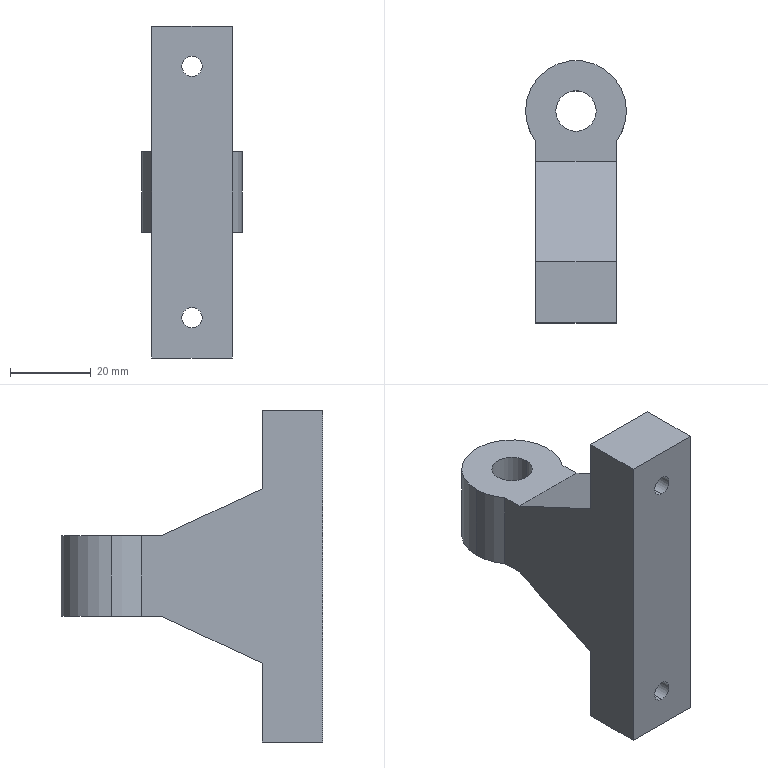Part | SolidWorks | features ICE 2, 3DProfileFeature 1, Extrusion 1, HoleWzd 1, MirrorPattern 1 | 1 solid | 20 faces | box 25 x 65 x 82.337 mm | volume 48790 mm3 | plane 11 | cylinder 9 | commonest cylinder face diameters 5 x4 25 x3 10 x2
STEP:
#1=CARTESIAN_POINT('',(0.,-52.5,28.668));
#2=VERTEX_POINT('',#1);
#3=CARTESIAN_POINT('',(0.,-52.5,33.668));
#4=VERTEX_POINT('',#3);
#5=CARTESIAN_POINT('',(0.,-52.5,31.168));
#6=DIRECTION('',(0.,1.,0.));
#7=DIRECTION('',(0.,0.,1.));
#8=AXIS2_PLACEMENT_3D('',#5,#6,#7);
#9=CIRCLE('',#8,2.5);
#10=EDGE_CURVE('',#2,#4,#9,.T.);
#11=ORIENTED_EDGE('',*,*,#10,.F.);
#12=CARTESIAN_POINT('',(0.,-37.5,28.668));
#13=VERTEX_POINT('',#12);
#14=CARTESIAN_POINT('',(0.,-37.5,28.668));
#15=DIRECTION('',(0.,1.,0.));
#16=VECTOR('',#15,1000.);
#17=LINE('',#14,#16);
#18=EDGE_CURVE('',#2,#13,#17,.T.);
#19=ORIENTED_EDGE('',*,*,#18,.T.);
#20=CARTESIAN_POINT('',(0.,-37.5,33.668));
#21=VERTEX_POINT('',#20);
#22=CARTESIAN_POINT('',(0.,-37.5,31.168));
#23=DIRECTION('',(0.,1.,0.));
#24=DIRECTION('',(0.,0.,1.));
#25=AXIS2_PLACEMENT_3D('',#22,#23,#24);
#26=CIRCLE('',#25,2.5);
#27=EDGE_CURVE('',#13,#21,#26,.T.);
#28=ORIENTED_EDGE('',*,*,#27,.T.);
#29=CARTESIAN_POINT('',(0.,-37.5,33.668));
#30=DIRECTION('',(0.,1.,0.));
#31=VECTOR('',#30,1000.);
#32=LINE('',#29,#31);
#33=EDGE_CURVE('',#4,#21,#32,.T.);
#34=ORIENTED_EDGE('',*,*,#33,.F.);
#35=EDGE_LOOP('',(#11,#19,#28,#34));
#36=FACE_OUTER_BOUND('',#35,.T.);
#37=CARTESIAN_POINT('',(0.,-37.5,31.168));
#38=DIRECTION('',(0.,1.,0.));
#39=DIRECTION('',(0.,0.,1.));
#40=AXIS2_PLACEMENT_3D('',#37,#38,#39);
#41=CYLINDRICAL_SURFACE('',#40,2.5);
#42=ADVANCED_FACE('',(#36),#41,.F.);
#43=CARTESIAN_POINT('',(0.,-52.5,-33.668));
#44=VERTEX_POINT('',#43);
#45=CARTESIAN_POINT('',(0.,-52.5,-28.668));
#46=VERTEX_POINT('',#45);
#47=CARTESIAN_POINT('',(0.,-52.5,-31.168));
#48=DIRECTION('',(0.,1.,0.));
#49=DIRECTION('',(0.,0.,1.));
#50=AXIS2_PLACEMENT_3D('',#47,#48,#49);
#51=CIRCLE('',#50,2.5);
#52=EDGE_CURVE('',#44,#46,#51,.T.);
#53=ORIENTED_EDGE('',*,*,#52,.F.);
#54=CARTESIAN_POINT('',(0.,-37.5,-33.668));
#55=VERTEX_POINT('',#54);
#56=CARTESIAN_POINT('',(0.,-37.5,-33.668));
#57=DIRECTION('',(0.,1.,0.));
#58=VECTOR('',#57,1000.);
#59=LINE('',#56,#58);
#60=EDGE_CURVE('',#44,#55,#59,.T.);
#61=ORIENTED_EDGE('',*,*,#60,.T.);
#62=CARTESIAN_POINT('',(0.,-37.5,-28.668));
#63=VERTEX_POINT('',#62);
#64=CARTESIAN_POINT('',(0.,-37.5,-31.168));
#65=DIRECTION('',(0.,1.,0.));
#66=DIRECTION('',(0.,0.,1.));
#67=AXIS2_PLACEMENT_3D('',#64,#65,#66);
#68=CIRCLE('',#67,2.5);
#69=EDGE_CURVE('',#55,#63,#68,.T.);
#70=ORIENTED_EDGE('',*,*,#69,.T.);
#71=CARTESIAN_POINT('',(0.,-37.5,-28.668));
#72=DIRECTION('',(0.,1.,0.));
#73=VECTOR('',#72,1000.);
#74=LINE('',#71,#73);
#75=EDGE_CURVE('',#46,#63,#74,.T.);
#76=ORIENTED_EDGE('',*,*,#75,.F.);
#77=EDGE_LOOP('',(#53,#61,#70,#76));
#78=FACE_OUTER_BOUND('',#77,.T.);
#79=CARTESIAN_POINT('',(0.,-37.5,-31.168));
#80=DIRECTION('',(0.,1.,0.));
#81=DIRECTION('',(0.,0.,1.));
#82=AXIS2_PLACEMENT_3D('',#79,#80,#81);
#83=CYLINDRICAL_SURFACE('',#82,2.5);
#84=ADVANCED_FACE('',(#78),#83,.F.);
#85=CARTESIAN_POINT('',(-5.,0.,10.));
#86=VERTEX_POINT('',#85);
#87=CARTESIAN_POINT('',(5.,0.,10.));
#88=VERTEX_POINT('',#87);
#89=CARTESIAN_POINT('',(0.,0.,10.));
#90=DIRECTION('',(0.,0.,1.));
#91=DIRECTION('',(1.,0.,0.));
#92=AXIS2_PLACEMENT_3D('',#89,#90,#91);
#93=CIRCLE('',#92,5.);
#94=EDGE_CURVE('',#86,#88,#93,.T.);
#95=ORIENTED_EDGE('',*,*,#94,.T.);
#96=CARTESIAN_POINT('',(5.,0.,-10.));
#97=VERTEX_POINT('',#96);
#98=CARTESIAN_POINT('',(5.,0.,10.));
#99=DIRECTION('',(0.,0.,-1.));
#100=VECTOR('',#99,1000.);
#101=LINE('',#98,#100);
#102=EDGE_CURVE('',#88,#97,#101,.T.);
#103=ORIENTED_EDGE('',*,*,#102,.T.);
#104=CARTESIAN_POINT('',(-5.,0.,-10.));
#105=VERTEX_POINT('',#104);
#106=CARTESIAN_POINT('',(0.,0.,-10.));
#107=DIRECTION('',(0.,0.,1.));
#108=DIRECTION('',(1.,0.,0.));
#109=AXIS2_PLACEMENT_3D('',#106,#107,#108);
#110=CIRCLE('',#109,5.);
#111=EDGE_CURVE('',#105,#97,#110,.T.);
#112=ORIENTED_EDGE('',*,*,#111,.F.);
#113=CARTESIAN_POINT('',(-5.,0.,10.));
#114=DIRECTION('',(0.,0.,-1.));
#115=VECTOR('',#114,1000.);
#116=LINE('',#113,#115);
#117=EDGE_CURVE('',#86,#105,#116,.T.);
#118=ORIENTED_EDGE('',*,*,#117,.F.);
#119=EDGE_LOOP('',(#95,#103,#112,#118));
#120=FACE_OUTER_BOUND('',#119,.T.);
#121=CARTESIAN_POINT('',(0.,0.,10.));
#122=DIRECTION('',(0.,0.,-1.));
#123=DIRECTION('',(-1.,0.,0.));
#124=AXIS2_PLACEMENT_3D('',#121,#122,#123);
#125=CYLINDRICAL_SURFACE('',#124,5.);
#126=ADVANCED_FACE('',(#120),#125,.F.);
#127=CARTESIAN_POINT('',(12.5,0.,10.));
#128=VERTEX_POINT('',#127);
#129=CARTESIAN_POINT('',(-12.5,0.,10.));
#130=VERTEX_POINT('',#129);
#131=CARTESIAN_POINT('',(0.,0.,10.));
#132=DIRECTION('',(0.,0.,1.));
#133=DIRECTION('',(1.,0.,0.));
#134=AXIS2_PLACEMENT_3D('',#131,#132,#133);
#135=CIRCLE('',#134,12.5);
#136=EDGE_CURVE('',#128,#130,#135,.T.);
#137=ORIENTED_EDGE('',*,*,#136,.F.);
#138=CARTESIAN_POINT('',(12.5,0.,-10.));
#139=VERTEX_POINT('',#138);
#140=CARTESIAN_POINT('',(12.5,0.,10.));
#141=DIRECTION('',(0.,0.,-1.));
#142=VECTOR('',#141,1000.);
#143=LINE('',#140,#142);
#144=EDGE_CURVE('',#128,#139,#143,.T.);
#145=ORIENTED_EDGE('',*,*,#144,.T.);
#146=CARTESIAN_POINT('',(-12.5,0.,-10.));
#147=VERTEX_POINT('',#146);
#148=CARTESIAN_POINT('',(0.,0.,-10.));
#149=DIRECTION('',(0.,0.,1.));
#150=DIRECTION('',(1.,0.,0.));
#151=AXIS2_PLACEMENT_3D('',#148,#149,#150);
#152=CIRCLE('',#151,12.5);
#153=EDGE_CURVE('',#139,#147,#152,.T.);
#154=ORIENTED_EDGE('',*,*,#153,.T.);
#155=CARTESIAN_POINT('',(-12.5,0.,10.));
#156=DIRECTION('',(0.,0.,-1.));
#157=VECTOR('',#156,1000.);
#158=LINE('',#155,#157);
#159=EDGE_CURVE('',#130,#147,#158,.T.);
#160=ORIENTED_EDGE('',*,*,#159,.F.);
#161=EDGE_LOOP('',(#137,#145,#154,#160));
#162=FACE_OUTER_BOUND('',#161,.T.);
#163=CARTESIAN_POINT('',(0.,0.,10.));
#164=DIRECTION('',(0.,0.,-1.));
#165=DIRECTION('',(-1.,0.,0.));
#166=AXIS2_PLACEMENT_3D('',#163,#164,#165);
#167=CYLINDRICAL_SURFACE('',#166,12.5);
#168=ADVANCED_FACE('',(#162),#167,.T.);
#169=CARTESIAN_POINT('',(-10.,-7.5,10.));
#170=VERTEX_POINT('',#169);
#171=CARTESIAN_POINT('',(0.,0.,10.));
#172=DIRECTION('',(0.,0.,1.));
#173=DIRECTION('',(1.,0.,0.));
#174=AXIS2_PLACEMENT_3D('',#171,#172,#173);
#175=CIRCLE('',#174,12.5);
#176=EDGE_CURVE('',#130,#170,#175,.T.);
#177=ORIENTED_EDGE('',*,*,#176,.F.);
#178=ORIENTED_EDGE('',*,*,#159,.T.);
#179=CARTESIAN_POINT('',(-10.,-7.5,-10.));
#180=VERTEX_POINT('',#179);
#181=CARTESIAN_POINT('',(0.,0.,-10.));
#182=DIRECTION('',(0.,0.,1.));
#183=DIRECTION('',(1.,0.,0.));
#184=AXIS2_PLACEMENT_3D('',#181,#182,#183);
#185=CIRCLE('',#184,12.5);
#186=EDGE_CURVE('',#147,#180,#185,.T.);
#187=ORIENTED_EDGE('',*,*,#186,.T.);
#188=CARTESIAN_POINT('',(-10.,-7.5,10.));
#189=DIRECTION('',(0.,0.,1.));
#190=VECTOR('',#189,1000.);
#191=LINE('',#188,#190);
#192=EDGE_CURVE('',#180,#170,#191,.T.);
#193=ORIENTED_EDGE('',*,*,#192,.T.);
#194=EDGE_LOOP('',(#177,#178,#187,#193));
#195=FACE_OUTER_BOUND('',#194,.T.);
#196=CARTESIAN_POINT('',(0.,0.,10.));
#197=DIRECTION('',(0.,0.,-1.));
#198=DIRECTION('',(-1.,0.,0.));
#199=AXIS2_PLACEMENT_3D('',#196,#197,#198);
#200=CYLINDRICAL_SURFACE('',#199,12.5);
#201=ADVANCED_FACE('',(#195),#200,.T.);
#202=CARTESIAN_POINT('',(-10.,-37.5,-41.168));
#203=VERTEX_POINT('',#202);
#204=CARTESIAN_POINT('',(-10.,-37.5,-21.658));
#205=VERTEX_POINT('',#204);
#206=CARTESIAN_POINT('',(-10.,-37.5,-21.658));
#207=DIRECTION('',(0.,0.,1.));
#208=VECTOR('',#207,1000.);
#209=LINE('',#206,#208);
#210=EDGE_CURVE('',#203,#205,#209,.T.);
#211=ORIENTED_EDGE('',*,*,#210,.T.);
#212=CARTESIAN_POINT('',(10.,-37.5,-21.658));
#213=VERTEX_POINT('',#212);
#214=CARTESIAN_POINT('',(10.,-37.5,-21.658));
#215=DIRECTION('',(-1.,0.,0.));
#216=VECTOR('',#215,1000.);
#217=LINE('',#214,#216);
#218=EDGE_CURVE('',#213,#205,#217,.T.);
#219=ORIENTED_EDGE('',*,*,#218,.F.);
#220=CARTESIAN_POINT('',(10.,-37.5,-41.168));
#221=VERTEX_POINT('',#220);
#222=CARTESIAN_POINT('',(10.,-37.5,-21.658));
#223=DIRECTION('',(0.,0.,1.));
#224=VECTOR('',#223,1000.);
#225=LINE('',#222,#224);
#226=EDGE_CURVE('',#221,#213,#225,.T.);
#227=ORIENTED_EDGE('',*,*,#226,.F.);
#228=CARTESIAN_POINT('',(10.,-37.5,-41.168));
#229=DIRECTION('',(-1.,0.,0.));
#230=VECTOR('',#229,1000.);
#231=LINE('',#228,#230);
#232=EDGE_CURVE('',#221,#203,#231,.T.);
#233=ORIENTED_EDGE('',*,*,#232,.T.);
#234=EDGE_LOOP('',(#211,#219,#227,#233));
#235=FACE_OUTER_BOUND('',#234,.T.);
#236=CARTESIAN_POINT('',(0.,-37.5,-31.168));
#237=DIRECTION('',(0.,1.,0.));
#238=DIRECTION('',(0.,0.,1.));
#239=AXIS2_PLACEMENT_3D('',#236,#237,#238);
#240=CIRCLE('',#239,2.5);
#241=EDGE_CURVE('',#63,#55,#240,.T.);
#242=ORIENTED_EDGE('',*,*,#241,.F.);
#243=ORIENTED_EDGE('',*,*,#69,.F.);
#244=EDGE_LOOP('',(#242,#243));
#245=FACE_BOUND('',#244,.T.);
#246=CARTESIAN_POINT('',(10.,-37.5,-21.658));
#247=DIRECTION('',(0.,-1.,0.));
#248=DIRECTION('',(0.,0.,-1.));
#249=AXIS2_PLACEMENT_3D('',#246,#247,#248);
#250=PLANE('',#249);
#251=ADVANCED_FACE('',(#235,#245),#250,.F.);
#252=ORIENTED_EDGE('',*,*,#144,.F.);
#253=CARTESIAN_POINT('',(10.,-7.5,10.));
#254=VERTEX_POINT('',#253);
#255=CARTESIAN_POINT('',(0.,0.,10.));
#256=DIRECTION('',(0.,0.,1.));
#257=DIRECTION('',(1.,0.,0.));
#258=AXIS2_PLACEMENT_3D('',#255,#256,#257);
#259=CIRCLE('',#258,12.5);
#260=EDGE_CURVE('',#254,#128,#259,.T.);
#261=ORIENTED_EDGE('',*,*,#260,.F.);
#262=CARTESIAN_POINT('',(10.,-7.5,-10.));
#263=VERTEX_POINT('',#262);
#264=CARTESIAN_POINT('',(10.,-7.5,10.));
#265=DIRECTION('',(0.,0.,-1.));
#266=VECTOR('',#265,1000.);
#267=LINE('',#264,#266);
#268=EDGE_CURVE('',#254,#263,#267,.T.);
#269=ORIENTED_EDGE('',*,*,#268,.T.);
#270=CARTESIAN_POINT('',(0.,0.,-10.));
#271=DIRECTION('',(0.,0.,1.));
#272=DIRECTION('',(1.,0.,0.));
#273=AXIS2_PLACEMENT_3D('',#270,#271,#272);
#274=CIRCLE('',#273,12.5);
#275=EDGE_CURVE('',#263,#139,#274,.T.);
#276=ORIENTED_EDGE('',*,*,#275,.T.);
#277=EDGE_LOOP('',(#252,#261,#269,#276));
#278=FACE_OUTER_BOUND('',#277,.T.);
#279=CARTESIAN_POINT('',(0.,0.,10.));
#280=DIRECTION('',(0.,0.,-1.));
#281=DIRECTION('',(-1.,0.,0.));
#282=AXIS2_PLACEMENT_3D('',#279,#280,#281);
#283=CYLINDRICAL_SURFACE('',#282,12.5);
#284=ADVANCED_FACE('',(#278),#283,.T.);
#285=CARTESIAN_POINT('',(-10.,-12.5,10.));
#286=VERTEX_POINT('',#285);
#287=CARTESIAN_POINT('',(10.,-12.5,10.));
#288=VERTEX_POINT('',#287);
#289=CARTESIAN_POINT('',(-10.,-12.5,10.));
#290=DIRECTION('',(1.,0.,0.));
#291=VECTOR('',#290,1000.);
#292=LINE('',#289,#291);
#293=EDGE_CURVE('',#286,#288,#292,.T.);
#294=ORIENTED_EDGE('',*,*,#293,.T.);
#295=CARTESIAN_POINT('',(10.,12.501,10.));
#296=DIRECTION('',(0.,-1.,0.));
#297=VECTOR('',#296,1000.);
#298=LINE('',#295,#297);
#299=EDGE_CURVE('',#254,#288,#298,.T.);
#300=ORIENTED_EDGE('',*,*,#299,.F.);
#301=ORIENTED_EDGE('',*,*,#260,.T.);
#302=ORIENTED_EDGE('',*,*,#136,.T.);
#303=ORIENTED_EDGE('',*,*,#176,.T.);
#304=CARTESIAN_POINT('',(-10.,12.501,10.));
#305=DIRECTION('',(0.,-1.,0.));
#306=VECTOR('',#305,1000.);
#307=LINE('',#304,#306);
#308=EDGE_CURVE('',#170,#286,#307,.T.);
#309=ORIENTED_EDGE('',*,*,#308,.T.);
#310=EDGE_LOOP('',(#294,#300,#301,#302,#303,#309));
#311=FACE_OUTER_BOUND('',#310,.T.);
#312=ORIENTED_EDGE('',*,*,#94,.F.);
#313=CARTESIAN_POINT('',(0.,0.,10.));
#314=DIRECTION('',(0.,0.,1.));
#315=DIRECTION('',(1.,0.,0.));
#316=AXIS2_PLACEMENT_3D('',#313,#314,#315);
#317=CIRCLE('',#316,5.);
#318=EDGE_CURVE('',#88,#86,#317,.T.);
#319=ORIENTED_EDGE('',*,*,#318,.F.);
#320=EDGE_LOOP('',(#312,#319));
#321=FACE_BOUND('',#320,.T.);
#322=CARTESIAN_POINT('',(0.,0.,10.));
#323=DIRECTION('',(0.,0.,1.));
#324=DIRECTION('',(1.,0.,0.));
#325=AXIS2_PLACEMENT_3D('',#322,#323,#324);
#326=PLANE('',#325);
#327=ADVANCED_FACE('',(#311,#321),#326,.T.);
#328=ORIENTED_EDGE('',*,*,#275,.F.);
#329=CARTESIAN_POINT('',(10.,-12.5,-10.));
#330=VERTEX_POINT('',#329);
#331=CARTESIAN_POINT('',(10.,12.501,-10.));
#332=DIRECTION('',(0.,-1.,0.));
#333=VECTOR('',#332,1000.);
#334=LINE('',#331,#333);
#335=EDGE_CURVE('',#263,#330,#334,.T.);
#336=ORIENTED_EDGE('',*,*,#335,.T.);
#337=CARTESIAN_POINT('',(-10.,-12.5,-10.));
#338=VERTEX_POINT('',#337);
#339=CARTESIAN_POINT('',(10.,-12.5,-10.));
#340=DIRECTION('',(-1.,0.,0.));
#341=VECTOR('',#340,1000.);
#342=LINE('',#339,#341);
#343=EDGE_CURVE('',#330,#338,#342,.T.);
#344=ORIENTED_EDGE('',*,*,#343,.T.);
#345=CARTESIAN_POINT('',(-10.,12.501,-10.));
#346=DIRECTION('',(0.,-1.,0.));
#347=VECTOR('',#346,1000.);
#348=LINE('',#345,#347);
#349=EDGE_CURVE('',#180,#338,#348,.T.);
#350=ORIENTED_EDGE('',*,*,#349,.F.);
#351=ORIENTED_EDGE('',*,*,#186,.F.);
#352=ORIENTED_EDGE('',*,*,#153,.F.);
#353=EDGE_LOOP('',(#328,#336,#344,#350,#351,#352));
#354=FACE_OUTER_BOUND('',#353,.T.);
#355=ORIENTED_EDGE('',*,*,#111,.T.);
#356=CARTESIAN_POINT('',(0.,0.,-10.));
#357=DIRECTION('',(0.,0.,1.));
#358=DIRECTION('',(1.,0.,0.));
#359=AXIS2_PLACEMENT_3D('',#356,#357,#358);
#360=CIRCLE('',#359,5.);
#361=EDGE_CURVE('',#97,#105,#360,.T.);
#362=ORIENTED_EDGE('',*,*,#361,.T.);
#363=EDGE_LOOP('',(#355,#362));
#364=FACE_BOUND('',#363,.T.);
#365=CARTESIAN_POINT('',(0.,0.,-10.));
#366=DIRECTION('',(0.,0.,1.));
#367=DIRECTION('',(1.,0.,0.));
#368=AXIS2_PLACEMENT_3D('',#365,#366,#367);
#369=PLANE('',#368);
#370=ADVANCED_FACE('',(#354,#364),#369,.F.);
#371=ORIENTED_EDGE('',*,*,#102,.F.);
#372=ORIENTED_EDGE('',*,*,#318,.T.);
#373=ORIENTED_EDGE('',*,*,#117,.T.);
#374=ORIENTED_EDGE('',*,*,#361,.F.);
#375=EDGE_LOOP('',(#371,#372,#373,#374));
#376=FACE_OUTER_BOUND('',#375,.T.);
#377=CARTESIAN_POINT('',(0.,0.,10.));
#378=DIRECTION('',(0.,0.,-1.));
#379=DIRECTION('',(-1.,0.,0.));
#380=AXIS2_PLACEMENT_3D('',#377,#378,#379);
#381=CYLINDRICAL_SURFACE('',#380,5.);
#382=ADVANCED_FACE('',(#376),#381,.F.);
#383=ORIENTED_EDGE('',*,*,#192,.F.);
#384=ORIENTED_EDGE('',*,*,#349,.T.);
#385=CARTESIAN_POINT('',(-10.,-12.5,-10.));
#386=DIRECTION('',(0.,0.9063,0.4226));
#387=VECTOR('',#386,1000.);
#388=LINE('',#385,#387);
#389=EDGE_CURVE('',#205,#338,#388,.T.);
#390=ORIENTED_EDGE('',*,*,#389,.F.);
#391=ORIENTED_EDGE('',*,*,#210,.F.);
#392=CARTESIAN_POINT('',(-10.,-52.5,-41.168));
#393=VERTEX_POINT('',#392);
#394=CARTESIAN_POINT('',(-10.,-37.5,-41.168));
#395=DIRECTION('',(0.,1.,0.));
#396=VECTOR('',#395,1000.);
#397=LINE('',#394,#396);
#398=EDGE_CURVE('',#393,#203,#397,.T.);
#399=ORIENTED_EDGE('',*,*,#398,.F.);
#400=CARTESIAN_POINT('',(-10.,-52.5,41.168));
#401=VERTEX_POINT('',#400);
#402=CARTESIAN_POINT('',(-10.,-52.5,-41.168));
#403=DIRECTION('',(0.,0.,-1.));
#404=VECTOR('',#403,1000.);
#405=LINE('',#402,#404);
#406=EDGE_CURVE('',#401,#393,#405,.T.);
#407=ORIENTED_EDGE('',*,*,#406,.F.);
#408=CARTESIAN_POINT('',(-10.,-37.5,41.168));
#409=VERTEX_POINT('',#408);
#410=CARTESIAN_POINT('',(-10.,-37.5,41.168));
#411=DIRECTION('',(0.,-1.,0.));
#412=VECTOR('',#411,1000.);
#413=LINE('',#410,#412);
#414=EDGE_CURVE('',#409,#401,#413,.T.);
#415=ORIENTED_EDGE('',*,*,#414,.F.);
#416=CARTESIAN_POINT('',(-10.,-37.5,21.658));
#417=VERTEX_POINT('',#416);
#418=CARTESIAN_POINT('',(-10.,-37.5,21.658));
#419=DIRECTION('',(0.,0.,1.));
#420=VECTOR('',#419,1000.);
#421=LINE('',#418,#420);
#422=EDGE_CURVE('',#417,#409,#421,.T.);
#423=ORIENTED_EDGE('',*,*,#422,.F.);
#424=CARTESIAN_POINT('',(-10.,-12.5,10.));
#425=DIRECTION('',(0.,-0.9063,0.4226));
#426=VECTOR('',#425,1000.);
#427=LINE('',#424,#426);
#428=EDGE_CURVE('',#286,#417,#427,.T.);
#429=ORIENTED_EDGE('',*,*,#428,.F.);
#430=ORIENTED_EDGE('',*,*,#308,.F.);
#431=EDGE_LOOP('',(#383,#384,#390,#391,#399,#407,#415,#423,#429,#430));
#432=FACE_OUTER_BOUND('',#431,.T.);
#433=CARTESIAN_POINT('',(-10.,12.501,-10.));
#434=DIRECTION('',(1.,0.,0.));
#435=DIRECTION('',(0.,0.,-1.));
#436=AXIS2_PLACEMENT_3D('',#433,#434,#435);
#437=PLANE('',#436);
#438=ADVANCED_FACE('',(#432),#437,.F.);
#439=ORIENTED_EDGE('',*,*,#428,.T.);
#440=CARTESIAN_POINT('',(10.,-37.5,21.658));
#441=VERTEX_POINT('',#440);
#442=CARTESIAN_POINT('',(10.,-37.5,21.658));
#443=DIRECTION('',(-1.,0.,0.));
#444=VECTOR('',#443,1000.);
#445=LINE('',#442,#444);
#446=EDGE_CURVE('',#441,#417,#445,.T.);
#447=ORIENTED_EDGE('',*,*,#446,.F.);
#448=CARTESIAN_POINT('',(10.,-12.5,10.));
#449=DIRECTION('',(0.,-0.9063,0.4226));
#450=VECTOR('',#449,1000.);
#451=LINE('',#448,#450);
#452=EDGE_CURVE('',#288,#441,#451,.T.);
#453=ORIENTED_EDGE('',*,*,#452,.F.);
#454=ORIENTED_EDGE('',*,*,#293,.F.);
#455=EDGE_LOOP('',(#439,#447,#453,#454));
#456=FACE_OUTER_BOUND('',#455,.T.);
#457=CARTESIAN_POINT('',(10.,-12.5,10.));
#458=DIRECTION('',(0.,-0.4226,-0.9063));
#459=DIRECTION('',(0.,0.9063,-0.4226));
#460=AXIS2_PLACEMENT_3D('',#457,#458,#459);
#461=PLANE('',#460);
#462=ADVANCED_FACE('',(#456),#461,.F.);
#463=CARTESIAN_POINT('',(0.,-37.5,31.168));
#464=DIRECTION('',(0.,1.,0.));
#465=DIRECTION('',(0.,0.,1.));
#466=AXIS2_PLACEMENT_3D('',#463,#464,#465);
#467=CIRCLE('',#466,2.5);
#468=EDGE_CURVE('',#21,#13,#467,.T.);
#469=ORIENTED_EDGE('',*,*,#468,.F.);
#470=ORIENTED_EDGE('',*,*,#27,.F.);
#471=EDGE_LOOP('',(#469,#470));
#472=FACE_BOUND('',#471,.T.);
#473=ORIENTED_EDGE('',*,*,#422,.T.);
#474=CARTESIAN_POINT('',(10.,-37.5,41.168));
#475=VERTEX_POINT('',#474);
#476=CARTESIAN_POINT('',(10.,-37.5,41.168));
#477=DIRECTION('',(-1.,0.,0.));
#478=VECTOR('',#477,1000.);
#479=LINE('',#476,#478);
#480=EDGE_CURVE('',#475,#409,#479,.T.);
#481=ORIENTED_EDGE('',*,*,#480,.F.);
#482=CARTESIAN_POINT('',(10.,-37.5,21.658));
#483=DIRECTION('',(0.,0.,1.));
#484=VECTOR('',#483,1000.);
#485=LINE('',#482,#484);
#486=EDGE_CURVE('',#441,#475,#485,.T.);
#487=ORIENTED_EDGE('',*,*,#486,.F.);
#488=ORIENTED_EDGE('',*,*,#446,.T.);
#489=EDGE_LOOP('',(#473,#481,#487,#488));
#490=FACE_OUTER_BOUND('',#489,.T.);
#491=CARTESIAN_POINT('',(10.,-37.5,21.658));
#492=DIRECTION('',(0.,-1.,0.));
#493=DIRECTION('',(0.,0.,-1.));
#494=AXIS2_PLACEMENT_3D('',#491,#492,#493);
#495=PLANE('',#494);
#496=ADVANCED_FACE('',(#472,#490),#495,.F.);
#497=ORIENTED_EDGE('',*,*,#414,.T.);
#498=CARTESIAN_POINT('',(10.,-52.5,41.168));
#499=VERTEX_POINT('',#498);
#500=CARTESIAN_POINT('',(10.,-52.5,41.168));
#501=DIRECTION('',(-1.,0.,0.));
#502=VECTOR('',#501,1000.);
#503=LINE('',#500,#502);
#504=EDGE_CURVE('',#499,#401,#503,.T.);
#505=ORIENTED_EDGE('',*,*,#504,.F.);
#506=CARTESIAN_POINT('',(10.,-37.5,41.168));
#507=DIRECTION('',(0.,-1.,0.));
#508=VECTOR('',#507,1000.);
#509=LINE('',#506,#508);
#510=EDGE_CURVE('',#475,#499,#509,.T.);
#511=ORIENTED_EDGE('',*,*,#510,.F.);
#512=ORIENTED_EDGE('',*,*,#480,.T.);
#513=EDGE_LOOP('',(#497,#505,#511,#512));
#514=FACE_OUTER_BOUND('',#513,.T.);
#515=CARTESIAN_POINT('',(10.,-37.5,41.168));
#516=DIRECTION('',(0.,0.,-1.));
#517=DIRECTION('',(-1.,0.,0.));
#518=AXIS2_PLACEMENT_3D('',#515,#516,#517);
#519=PLANE('',#518);
#520=ADVANCED_FACE('',(#514),#519,.F.);
#521=CARTESIAN_POINT('',(0.,-52.5,31.168));
#522=DIRECTION('',(0.,1.,0.));
#523=DIRECTION('',(0.,0.,1.));
#524=AXIS2_PLACEMENT_3D('',#521,#522,#523);
#525=CIRCLE('',#524,2.5);
#526=EDGE_CURVE('',#4,#2,#525,.T.);
#527=ORIENTED_EDGE('',*,*,#526,.T.);
#528=ORIENTED_EDGE('',*,*,#10,.T.);
#529=EDGE_LOOP('',(#527,#528));
#530=FACE_BOUND('',#529,.T.);
#531=CARTESIAN_POINT('',(0.,-52.5,-31.168));
#532=DIRECTION('',(0.,1.,0.));
#533=DIRECTION('',(0.,0.,1.));
#534=AXIS2_PLACEMENT_3D('',#531,#532,#533);
#535=CIRCLE('',#534,2.5);
#536=EDGE_CURVE('',#46,#44,#535,.T.);
#537=ORIENTED_EDGE('',*,*,#536,.T.);
#538=ORIENTED_EDGE('',*,*,#52,.T.);
#539=EDGE_LOOP('',(#537,#538));
#540=FACE_BOUND('',#539,.T.);
#541=ORIENTED_EDGE('',*,*,#406,.T.);
#542=CARTESIAN_POINT('',(10.,-52.5,-41.168));
#543=VERTEX_POINT('',#542);
#544=CARTESIAN_POINT('',(10.,-52.5,-41.168));
#545=DIRECTION('',(-1.,0.,0.));
#546=VECTOR('',#545,1000.);
#547=LINE('',#544,#546);
#548=EDGE_CURVE('',#543,#393,#547,.T.);
#549=ORIENTED_EDGE('',*,*,#548,.F.);
#550=CARTESIAN_POINT('',(10.,-52.5,-41.168));
#551=DIRECTION('',(0.,0.,-1.));
#552=VECTOR('',#551,1000.);
#553=LINE('',#550,#552);
#554=EDGE_CURVE('',#499,#543,#553,.T.);
#555=ORIENTED_EDGE('',*,*,#554,.F.);
#556=ORIENTED_EDGE('',*,*,#504,.T.);
#557=EDGE_LOOP('',(#541,#549,#555,#556));
#558=FACE_OUTER_BOUND('',#557,.T.);
#559=CARTESIAN_POINT('',(10.,-52.5,-41.168));
#560=DIRECTION('',(0.,1.,0.));
#561=DIRECTION('',(0.,0.,1.));
#562=AXIS2_PLACEMENT_3D('',#559,#560,#561);
#563=PLANE('',#562);
#564=ADVANCED_FACE('',(#530,#540,#558),#563,.F.);
#565=ORIENTED_EDGE('',*,*,#398,.T.);
#566=ORIENTED_EDGE('',*,*,#232,.F.);
#567=CARTESIAN_POINT('',(10.,-37.5,-41.168));
#568=DIRECTION('',(0.,1.,0.));
#569=VECTOR('',#568,1000.);
#570=LINE('',#567,#569);
#571=EDGE_CURVE('',#543,#221,#570,.T.);
#572=ORIENTED_EDGE('',*,*,#571,.F.);
#573=ORIENTED_EDGE('',*,*,#548,.T.);
#574=EDGE_LOOP('',(#565,#566,#572,#573));
#575=FACE_OUTER_BOUND('',#574,.T.);
#576=CARTESIAN_POINT('',(10.,-37.5,-41.168));
#577=DIRECTION('',(0.,0.,1.));
#578=DIRECTION('',(1.,0.,0.));
#579=AXIS2_PLACEMENT_3D('',#576,#577,#578);
#580=PLANE('',#579);
#581=ADVANCED_FACE('',(#575),#580,.F.);
#582=ORIENTED_EDGE('',*,*,#389,.T.);
#583=ORIENTED_EDGE('',*,*,#343,.F.);
#584=CARTESIAN_POINT('',(10.,-12.5,-10.));
#585=DIRECTION('',(0.,0.9063,0.4226));
#586=VECTOR('',#585,1000.);
#587=LINE('',#584,#586);
#588=EDGE_CURVE('',#213,#330,#587,.T.);
#589=ORIENTED_EDGE('',*,*,#588,.F.);
#590=ORIENTED_EDGE('',*,*,#218,.T.);
#591=EDGE_LOOP('',(#582,#583,#589,#590));
#592=FACE_OUTER_BOUND('',#591,.T.);
#593=CARTESIAN_POINT('',(10.,-12.5,-10.));
#594=DIRECTION('',(0.,-0.4226,0.9063));
#595=DIRECTION('',(0.,-0.9063,-0.4226));
#596=AXIS2_PLACEMENT_3D('',#593,#594,#595);
#597=PLANE('',#596);
#598=ADVANCED_FACE('',(#592),#597,.F.);
#599=ORIENTED_EDGE('',*,*,#588,.T.);
#600=ORIENTED_EDGE('',*,*,#335,.F.);
#601=ORIENTED_EDGE('',*,*,#268,.F.);
#602=ORIENTED_EDGE('',*,*,#299,.T.);
#603=ORIENTED_EDGE('',*,*,#452,.T.);
#604=ORIENTED_EDGE('',*,*,#486,.T.);
#605=ORIENTED_EDGE('',*,*,#510,.T.);
#606=ORIENTED_EDGE('',*,*,#554,.T.);
#607=ORIENTED_EDGE('',*,*,#571,.T.);
#608=ORIENTED_EDGE('',*,*,#226,.T.);
#609=EDGE_LOOP('',(#599,#600,#601,#602,#603,#604,#605,#606,#607,#608));
#610=FACE_OUTER_BOUND('',#609,.T.);
#611=CARTESIAN_POINT('',(10.,0.,0.));
#612=DIRECTION('',(-1.,0.,0.));
#613=DIRECTION('',(0.,0.,1.));
#614=AXIS2_PLACEMENT_3D('',#611,#612,#613);
#615=PLANE('',#614);
#616=ADVANCED_FACE('',(#610),#615,.F.);
#617=ORIENTED_EDGE('',*,*,#60,.F.);
#618=ORIENTED_EDGE('',*,*,#536,.F.);
#619=ORIENTED_EDGE('',*,*,#75,.T.);
#620=ORIENTED_EDGE('',*,*,#241,.T.);
#621=EDGE_LOOP('',(#617,#618,#619,#620));
#622=FACE_OUTER_BOUND('',#621,.T.);
#623=CARTESIAN_POINT('',(0.,-37.5,-31.168));
#624=DIRECTION('',(0.,1.,0.));
#625=DIRECTION('',(0.,0.,1.));
#626=AXIS2_PLACEMENT_3D('',#623,#624,#625);
#627=CYLINDRICAL_SURFACE('',#626,2.5);
#628=ADVANCED_FACE('',(#622),#627,.F.);
#629=ORIENTED_EDGE('',*,*,#18,.F.);
#630=ORIENTED_EDGE('',*,*,#526,.F.);
#631=ORIENTED_EDGE('',*,*,#33,.T.);
#632=ORIENTED_EDGE('',*,*,#468,.T.);
#633=EDGE_LOOP('',(#629,#630,#631,#632));
#634=FACE_OUTER_BOUND('',#633,.T.);
#635=CARTESIAN_POINT('',(0.,-37.5,31.168));
#636=DIRECTION('',(0.,1.,0.));
#637=DIRECTION('',(0.,0.,1.));
#638=AXIS2_PLACEMENT_3D('',#635,#636,#637);
#639=CYLINDRICAL_SURFACE('',#638,2.5);
#640=ADVANCED_FACE('',(#634),#639,.F.);
#641=CLOSED_SHELL('',(#42,#84,#126,#168,#201,#251,#284,#327,#370,#382,#438,#462,#496,#520,#564,#581,#598,#616,#628,#640));
#642=MANIFOLD_SOLID_BREP('',#641);
#643=CARTESIAN_POINT('',(0.,0.,0.));
#644=DIRECTION('',(0.,0.,1.));
#645=DIRECTION('',(1.,0.,0.));
#646=AXIS2_PLACEMENT_3D('',#643,#644,#645);
#647=(LENGTH_UNIT()NAMED_UNIT(*)SI_UNIT(.MILLI.,.METRE.));
#648=UNCERTAINTY_MEASURE_WITH_UNIT(LENGTH_MEASURE(0.00001),#647,'','');
#649=(NAMED_UNIT(*)PLANE_ANGLE_UNIT()SI_UNIT($,.RADIAN.));
#650=(NAMED_UNIT(*)SI_UNIT($,.STERADIAN.)SOLID_ANGLE_UNIT());
#651=(GEOMETRIC_REPRESENTATION_CONTEXT(3)GLOBAL_UNCERTAINTY_ASSIGNED_CONTEXT((#648))GLOBAL_UNIT_ASSIGNED_CONTEXT((#647,#649,#650))REPRESENTATION_CONTEXT('',''));
#652=ADVANCED_BREP_SHAPE_REPRESENTATION('',(#642,#646),#651);